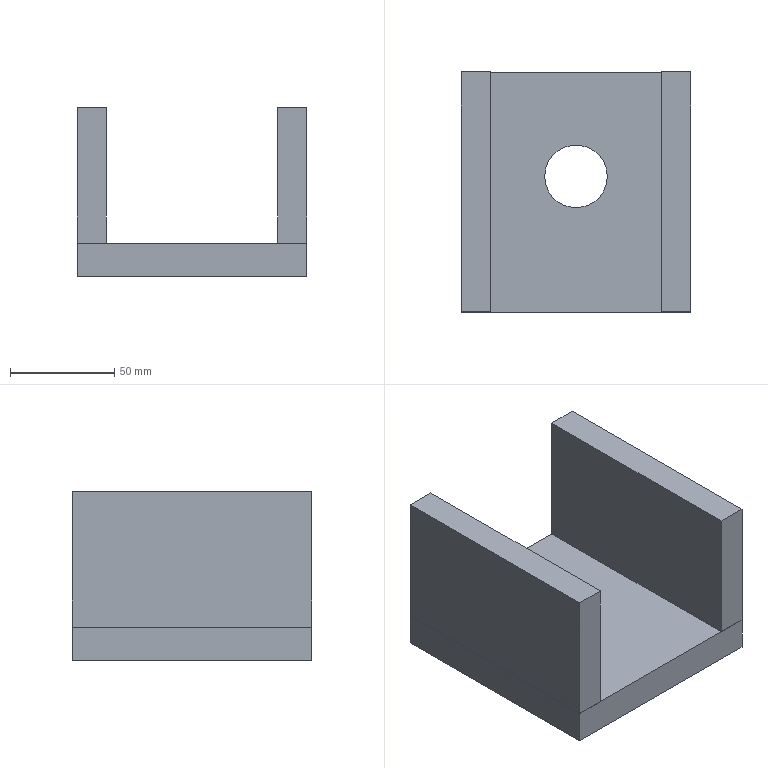Part | SolidWorks | features ICE 3, Extrusion 1, MirrorSolid 1, WeldmentFeature 1 | 3 solids | 20 faces | box 110 x 115 x 81 mm | volume 400390 mm3 | plane 18 | cylinder 2 | commonest cylinder face diameters 30 x2
STEP:
#1=CARTESIAN_POINT('',(-55.,50.,81.));
#2=VERTEX_POINT('',#1);
#3=CARTESIAN_POINT('',(-55.,50.,16.));
#4=VERTEX_POINT('',#3);
#5=CARTESIAN_POINT('',(-55.,50.,16.));
#6=DIRECTION('',(0.,0.,-1.));
#7=VECTOR('',#6,1000.);
#8=LINE('',#5,#7);
#9=EDGE_CURVE('',#2,#4,#8,.T.);
#10=ORIENTED_EDGE('',*,*,#9,.F.);
#11=CARTESIAN_POINT('',(-41.,50.,81.));
#12=VERTEX_POINT('',#11);
#13=CARTESIAN_POINT('',(-41.,50.,81.));
#14=DIRECTION('',(-1.,0.,0.));
#15=VECTOR('',#14,1000.);
#16=LINE('',#13,#15);
#17=EDGE_CURVE('',#12,#2,#16,.T.);
#18=ORIENTED_EDGE('',*,*,#17,.F.);
#19=CARTESIAN_POINT('',(-41.,50.,16.));
#20=VERTEX_POINT('',#19);
#21=CARTESIAN_POINT('',(-41.,50.,16.));
#22=DIRECTION('',(0.,0.,-1.));
#23=VECTOR('',#22,1000.);
#24=LINE('',#21,#23);
#25=EDGE_CURVE('',#12,#20,#24,.T.);
#26=ORIENTED_EDGE('',*,*,#25,.T.);
#27=CARTESIAN_POINT('',(-41.,50.,16.));
#28=DIRECTION('',(-1.,0.,0.));
#29=VECTOR('',#28,1000.);
#30=LINE('',#27,#29);
#31=EDGE_CURVE('',#20,#4,#30,.T.);
#32=ORIENTED_EDGE('',*,*,#31,.T.);
#33=EDGE_LOOP('',(#10,#18,#26,#32));
#34=FACE_OUTER_BOUND('',#33,.T.);
#35=CARTESIAN_POINT('',(-41.,50.,16.));
#36=DIRECTION('',(0.,1.,0.));
#37=DIRECTION('',(0.,0.,1.));
#38=AXIS2_PLACEMENT_3D('',#35,#36,#37);
#39=PLANE('',#38);
#40=ADVANCED_FACE('',(#34),#39,.T.);
#41=CARTESIAN_POINT('',(-55.,-65.,81.));
#42=VERTEX_POINT('',#41);
#43=CARTESIAN_POINT('',(-55.,50.,81.));
#44=DIRECTION('',(0.,1.,0.));
#45=VECTOR('',#44,1000.);
#46=LINE('',#43,#45);
#47=EDGE_CURVE('',#42,#2,#46,.T.);
#48=ORIENTED_EDGE('',*,*,#47,.F.);
#49=CARTESIAN_POINT('',(-41.,-65.,81.));
#50=VERTEX_POINT('',#49);
#51=CARTESIAN_POINT('',(-41.,-65.,81.));
#52=DIRECTION('',(-1.,0.,0.));
#53=VECTOR('',#52,1000.);
#54=LINE('',#51,#53);
#55=EDGE_CURVE('',#50,#42,#54,.T.);
#56=ORIENTED_EDGE('',*,*,#55,.F.);
#57=CARTESIAN_POINT('',(-41.,50.,81.));
#58=DIRECTION('',(0.,1.,0.));
#59=VECTOR('',#58,1000.);
#60=LINE('',#57,#59);
#61=EDGE_CURVE('',#50,#12,#60,.T.);
#62=ORIENTED_EDGE('',*,*,#61,.T.);
#63=ORIENTED_EDGE('',*,*,#17,.T.);
#64=EDGE_LOOP('',(#48,#56,#62,#63));
#65=FACE_OUTER_BOUND('',#64,.T.);
#66=CARTESIAN_POINT('',(-41.,50.,81.));
#67=DIRECTION('',(0.,0.,1.));
#68=DIRECTION('',(0.,-1.,0.));
#69=AXIS2_PLACEMENT_3D('',#66,#67,#68);
#70=PLANE('',#69);
#71=ADVANCED_FACE('',(#65),#70,.T.);
#72=CARTESIAN_POINT('',(-55.,-65.,16.));
#73=VERTEX_POINT('',#72);
#74=CARTESIAN_POINT('',(-55.,-65.,16.));
#75=DIRECTION('',(0.,0.,1.));
#76=VECTOR('',#75,1000.);
#77=LINE('',#74,#76);
#78=EDGE_CURVE('',#73,#42,#77,.T.);
#79=ORIENTED_EDGE('',*,*,#78,.F.);
#80=CARTESIAN_POINT('',(-41.,-65.,16.));
#81=VERTEX_POINT('',#80);
#82=CARTESIAN_POINT('',(-41.,-65.,16.));
#83=DIRECTION('',(-1.,0.,0.));
#84=VECTOR('',#83,1000.);
#85=LINE('',#82,#84);
#86=EDGE_CURVE('',#81,#73,#85,.T.);
#87=ORIENTED_EDGE('',*,*,#86,.F.);
#88=CARTESIAN_POINT('',(-41.,-65.,16.));
#89=DIRECTION('',(0.,0.,1.));
#90=VECTOR('',#89,1000.);
#91=LINE('',#88,#90);
#92=EDGE_CURVE('',#81,#50,#91,.T.);
#93=ORIENTED_EDGE('',*,*,#92,.T.);
#94=ORIENTED_EDGE('',*,*,#55,.T.);
#95=EDGE_LOOP('',(#79,#87,#93,#94));
#96=FACE_OUTER_BOUND('',#95,.T.);
#97=CARTESIAN_POINT('',(-41.,-65.,16.));
#98=DIRECTION('',(0.,-1.,0.));
#99=DIRECTION('',(0.,0.,-1.));
#100=AXIS2_PLACEMENT_3D('',#97,#98,#99);
#101=PLANE('',#100);
#102=ADVANCED_FACE('',(#96),#101,.T.);
#103=CARTESIAN_POINT('',(-55.,50.,16.));
#104=DIRECTION('',(0.,-1.,0.));
#105=VECTOR('',#104,1000.);
#106=LINE('',#103,#105);
#107=EDGE_CURVE('',#4,#73,#106,.T.);
#108=ORIENTED_EDGE('',*,*,#107,.F.);
#109=ORIENTED_EDGE('',*,*,#31,.F.);
#110=CARTESIAN_POINT('',(-41.,50.,16.));
#111=DIRECTION('',(0.,-1.,0.));
#112=VECTOR('',#111,1000.);
#113=LINE('',#110,#112);
#114=EDGE_CURVE('',#20,#81,#113,.T.);
#115=ORIENTED_EDGE('',*,*,#114,.T.);
#116=ORIENTED_EDGE('',*,*,#86,.T.);
#117=EDGE_LOOP('',(#108,#109,#115,#116));
#118=FACE_OUTER_BOUND('',#117,.T.);
#119=CARTESIAN_POINT('',(-41.,50.,16.));
#120=DIRECTION('',(0.,0.,-1.));
#121=DIRECTION('',(0.,1.,0.));
#122=AXIS2_PLACEMENT_3D('',#119,#120,#121);
#123=PLANE('',#122);
#124=ADVANCED_FACE('',(#118),#123,.T.);
#125=ORIENTED_EDGE('',*,*,#25,.F.);
#126=ORIENTED_EDGE('',*,*,#61,.F.);
#127=ORIENTED_EDGE('',*,*,#92,.F.);
#128=ORIENTED_EDGE('',*,*,#114,.F.);
#129=EDGE_LOOP('',(#125,#126,#127,#128));
#130=FACE_OUTER_BOUND('',#129,.T.);
#131=CARTESIAN_POINT('',(-41.,0.,0.));
#132=DIRECTION('',(1.,0.,0.));
#133=DIRECTION('',(0.,0.,-1.));
#134=AXIS2_PLACEMENT_3D('',#131,#132,#133);
#135=PLANE('',#134);
#136=ADVANCED_FACE('',(#130),#135,.T.);
#137=ORIENTED_EDGE('',*,*,#9,.T.);
#138=ORIENTED_EDGE('',*,*,#107,.T.);
#139=ORIENTED_EDGE('',*,*,#78,.T.);
#140=ORIENTED_EDGE('',*,*,#47,.T.);
#141=EDGE_LOOP('',(#137,#138,#139,#140));
#142=FACE_OUTER_BOUND('',#141,.T.);
#143=CARTESIAN_POINT('',(-55.,0.,0.));
#144=DIRECTION('',(1.,0.,0.));
#145=DIRECTION('',(0.,0.,-1.));
#146=AXIS2_PLACEMENT_3D('',#143,#144,#145);
#147=PLANE('',#146);
#148=ADVANCED_FACE('',(#142),#147,.F.);
#149=CLOSED_SHELL('',(#40,#71,#102,#124,#136,#148));
#150=MANIFOLD_SOLID_BREP('',#149);
#151=CARTESIAN_POINT('',(55.,50.,81.));
#152=VERTEX_POINT('',#151);
#153=CARTESIAN_POINT('',(55.,50.,16.));
#154=VERTEX_POINT('',#153);
#155=CARTESIAN_POINT('',(55.,50.,16.));
#156=DIRECTION('',(0.,0.,-1.));
#157=VECTOR('',#156,1000.);
#158=LINE('',#155,#157);
#159=EDGE_CURVE('',#152,#154,#158,.T.);
#160=ORIENTED_EDGE('',*,*,#159,.T.);
#161=CARTESIAN_POINT('',(41.,50.,16.));
#162=VERTEX_POINT('',#161);
#163=CARTESIAN_POINT('',(41.,50.,16.));
#164=DIRECTION('',(1.,0.,0.));
#165=VECTOR('',#164,1000.);
#166=LINE('',#163,#165);
#167=EDGE_CURVE('',#162,#154,#166,.T.);
#168=ORIENTED_EDGE('',*,*,#167,.F.);
#169=CARTESIAN_POINT('',(41.,50.,81.));
#170=VERTEX_POINT('',#169);
#171=CARTESIAN_POINT('',(41.,50.,16.));
#172=DIRECTION('',(0.,0.,-1.));
#173=VECTOR('',#172,1000.);
#174=LINE('',#171,#173);
#175=EDGE_CURVE('',#170,#162,#174,.T.);
#176=ORIENTED_EDGE('',*,*,#175,.F.);
#177=CARTESIAN_POINT('',(41.,50.,81.));
#178=DIRECTION('',(1.,0.,0.));
#179=VECTOR('',#178,1000.);
#180=LINE('',#177,#179);
#181=EDGE_CURVE('',#170,#152,#180,.T.);
#182=ORIENTED_EDGE('',*,*,#181,.T.);
#183=EDGE_LOOP('',(#160,#168,#176,#182));
#184=FACE_OUTER_BOUND('',#183,.T.);
#185=CARTESIAN_POINT('',(41.,50.,16.));
#186=DIRECTION('',(0.,1.,0.));
#187=DIRECTION('',(0.,0.,1.));
#188=AXIS2_PLACEMENT_3D('',#185,#186,#187);
#189=PLANE('',#188);
#190=ADVANCED_FACE('',(#184),#189,.T.);
#191=CARTESIAN_POINT('',(55.,-65.,81.));
#192=VERTEX_POINT('',#191);
#193=CARTESIAN_POINT('',(55.,50.,81.));
#194=DIRECTION('',(0.,1.,0.));
#195=VECTOR('',#194,1000.);
#196=LINE('',#193,#195);
#197=EDGE_CURVE('',#192,#152,#196,.T.);
#198=ORIENTED_EDGE('',*,*,#197,.T.);
#199=ORIENTED_EDGE('',*,*,#181,.F.);
#200=CARTESIAN_POINT('',(41.,-65.,81.));
#201=VERTEX_POINT('',#200);
#202=CARTESIAN_POINT('',(41.,50.,81.));
#203=DIRECTION('',(0.,1.,0.));
#204=VECTOR('',#203,1000.);
#205=LINE('',#202,#204);
#206=EDGE_CURVE('',#201,#170,#205,.T.);
#207=ORIENTED_EDGE('',*,*,#206,.F.);
#208=CARTESIAN_POINT('',(41.,-65.,81.));
#209=DIRECTION('',(1.,0.,0.));
#210=VECTOR('',#209,1000.);
#211=LINE('',#208,#210);
#212=EDGE_CURVE('',#201,#192,#211,.T.);
#213=ORIENTED_EDGE('',*,*,#212,.T.);
#214=EDGE_LOOP('',(#198,#199,#207,#213));
#215=FACE_OUTER_BOUND('',#214,.T.);
#216=CARTESIAN_POINT('',(41.,50.,81.));
#217=DIRECTION('',(0.,0.,1.));
#218=DIRECTION('',(0.,-1.,0.));
#219=AXIS2_PLACEMENT_3D('',#216,#217,#218);
#220=PLANE('',#219);
#221=ADVANCED_FACE('',(#215),#220,.T.);
#222=CARTESIAN_POINT('',(55.,-65.,16.));
#223=VERTEX_POINT('',#222);
#224=CARTESIAN_POINT('',(55.,-65.,16.));
#225=DIRECTION('',(0.,0.,1.));
#226=VECTOR('',#225,1000.);
#227=LINE('',#224,#226);
#228=EDGE_CURVE('',#223,#192,#227,.T.);
#229=ORIENTED_EDGE('',*,*,#228,.T.);
#230=ORIENTED_EDGE('',*,*,#212,.F.);
#231=CARTESIAN_POINT('',(41.,-65.,16.));
#232=VERTEX_POINT('',#231);
#233=CARTESIAN_POINT('',(41.,-65.,16.));
#234=DIRECTION('',(0.,0.,1.));
#235=VECTOR('',#234,1000.);
#236=LINE('',#233,#235);
#237=EDGE_CURVE('',#232,#201,#236,.T.);
#238=ORIENTED_EDGE('',*,*,#237,.F.);
#239=CARTESIAN_POINT('',(41.,-65.,16.));
#240=DIRECTION('',(1.,0.,0.));
#241=VECTOR('',#240,1000.);
#242=LINE('',#239,#241);
#243=EDGE_CURVE('',#232,#223,#242,.T.);
#244=ORIENTED_EDGE('',*,*,#243,.T.);
#245=EDGE_LOOP('',(#229,#230,#238,#244));
#246=FACE_OUTER_BOUND('',#245,.T.);
#247=CARTESIAN_POINT('',(41.,-65.,16.));
#248=DIRECTION('',(0.,-1.,0.));
#249=DIRECTION('',(0.,0.,-1.));
#250=AXIS2_PLACEMENT_3D('',#247,#248,#249);
#251=PLANE('',#250);
#252=ADVANCED_FACE('',(#246),#251,.T.);
#253=CARTESIAN_POINT('',(55.,50.,16.));
#254=DIRECTION('',(0.,-1.,0.));
#255=VECTOR('',#254,1000.);
#256=LINE('',#253,#255);
#257=EDGE_CURVE('',#154,#223,#256,.T.);
#258=ORIENTED_EDGE('',*,*,#257,.T.);
#259=ORIENTED_EDGE('',*,*,#243,.F.);
#260=CARTESIAN_POINT('',(41.,50.,16.));
#261=DIRECTION('',(0.,-1.,0.));
#262=VECTOR('',#261,1000.);
#263=LINE('',#260,#262);
#264=EDGE_CURVE('',#162,#232,#263,.T.);
#265=ORIENTED_EDGE('',*,*,#264,.F.);
#266=ORIENTED_EDGE('',*,*,#167,.T.);
#267=EDGE_LOOP('',(#258,#259,#265,#266));
#268=FACE_OUTER_BOUND('',#267,.T.);
#269=CARTESIAN_POINT('',(41.,50.,16.));
#270=DIRECTION('',(0.,0.,-1.));
#271=DIRECTION('',(0.,1.,0.));
#272=AXIS2_PLACEMENT_3D('',#269,#270,#271);
#273=PLANE('',#272);
#274=ADVANCED_FACE('',(#268),#273,.T.);
#275=ORIENTED_EDGE('',*,*,#175,.T.);
#276=ORIENTED_EDGE('',*,*,#264,.T.);
#277=ORIENTED_EDGE('',*,*,#237,.T.);
#278=ORIENTED_EDGE('',*,*,#206,.T.);
#279=EDGE_LOOP('',(#275,#276,#277,#278));
#280=FACE_OUTER_BOUND('',#279,.T.);
#281=CARTESIAN_POINT('',(41.,0.,0.));
#282=DIRECTION('',(-1.,0.,0.));
#283=DIRECTION('',(0.,0.,-1.));
#284=AXIS2_PLACEMENT_3D('',#281,#282,#283);
#285=PLANE('',#284);
#286=ADVANCED_FACE('',(#280),#285,.T.);
#287=ORIENTED_EDGE('',*,*,#159,.F.);
#288=ORIENTED_EDGE('',*,*,#197,.F.);
#289=ORIENTED_EDGE('',*,*,#228,.F.);
#290=ORIENTED_EDGE('',*,*,#257,.F.);
#291=EDGE_LOOP('',(#287,#288,#289,#290));
#292=FACE_OUTER_BOUND('',#291,.T.);
#293=CARTESIAN_POINT('',(55.,0.,0.));
#294=DIRECTION('',(-1.,0.,0.));
#295=DIRECTION('',(0.,0.,-1.));
#296=AXIS2_PLACEMENT_3D('',#293,#294,#295);
#297=PLANE('',#296);
#298=ADVANCED_FACE('',(#292),#297,.F.);
#299=CLOSED_SHELL('',(#190,#221,#252,#274,#286,#298));
#300=MANIFOLD_SOLID_BREP('',#299);
#301=CARTESIAN_POINT('',(-15.,0.,16.));
#302=VERTEX_POINT('',#301);
#303=CARTESIAN_POINT('',(15.,0.,16.));
#304=VERTEX_POINT('',#303);
#305=CARTESIAN_POINT('',(0.,0.,16.));
#306=DIRECTION('',(0.,0.,1.));
#307=DIRECTION('',(-1.,0.,0.));
#308=AXIS2_PLACEMENT_3D('',#305,#306,#307);
#309=CIRCLE('',#308,15.);
#310=EDGE_CURVE('',#302,#304,#309,.T.);
#311=ORIENTED_EDGE('',*,*,#310,.T.);
#312=CARTESIAN_POINT('',(15.,0.,0.));
#313=VERTEX_POINT('',#312);
#314=CARTESIAN_POINT('',(15.,0.,81.001));
#315=DIRECTION('',(0.,0.,-1.));
#316=VECTOR('',#315,1000.);
#317=LINE('',#314,#316);
#318=EDGE_CURVE('',#304,#313,#317,.T.);
#319=ORIENTED_EDGE('',*,*,#318,.T.);
#320=CARTESIAN_POINT('',(-15.,0.,0.));
#321=VERTEX_POINT('',#320);
#322=CARTESIAN_POINT('',(0.,0.,0.));
#323=DIRECTION('',(0.,0.,-1.));
#324=DIRECTION('',(-1.,0.,0.));
#325=AXIS2_PLACEMENT_3D('',#322,#323,#324);
#326=CIRCLE('',#325,15.);
#327=EDGE_CURVE('',#313,#321,#326,.T.);
#328=ORIENTED_EDGE('',*,*,#327,.T.);
#329=CARTESIAN_POINT('',(-15.,0.,81.001));
#330=DIRECTION('',(0.,0.,-1.));
#331=VECTOR('',#330,1000.);
#332=LINE('',#329,#331);
#333=EDGE_CURVE('',#302,#321,#332,.T.);
#334=ORIENTED_EDGE('',*,*,#333,.F.);
#335=EDGE_LOOP('',(#311,#319,#328,#334));
#336=FACE_OUTER_BOUND('',#335,.T.);
#337=CARTESIAN_POINT('',(0.,0.,81.001));
#338=DIRECTION('',(0.,0.,-1.));
#339=DIRECTION('',(-1.,0.,0.));
#340=AXIS2_PLACEMENT_3D('',#337,#338,#339);
#341=CYLINDRICAL_SURFACE('',#340,15.);
#342=ADVANCED_FACE('',(#336),#341,.F.);
#343=CARTESIAN_POINT('',(55.,-65.,0.));
#344=VERTEX_POINT('',#343);
#345=CARTESIAN_POINT('',(55.,50.,0.));
#346=VERTEX_POINT('',#345);
#347=CARTESIAN_POINT('',(55.,-50.,0.));
#348=DIRECTION('',(0.,1.,0.));
#349=VECTOR('',#348,1000.);
#350=LINE('',#347,#349);
#351=EDGE_CURVE('',#344,#346,#350,.T.);
#352=ORIENTED_EDGE('',*,*,#351,.T.);
#353=CARTESIAN_POINT('',(55.,50.,16.));
#354=VERTEX_POINT('',#353);
#355=CARTESIAN_POINT('',(55.,50.,16.));
#356=DIRECTION('',(0.,0.,-1.));
#357=VECTOR('',#356,1000.);
#358=LINE('',#355,#357);
#359=EDGE_CURVE('',#354,#346,#358,.T.);
#360=ORIENTED_EDGE('',*,*,#359,.F.);
#361=CARTESIAN_POINT('',(55.,-65.,16.));
#362=VERTEX_POINT('',#361);
#363=CARTESIAN_POINT('',(55.,-50.,16.));
#364=DIRECTION('',(0.,1.,0.));
#365=VECTOR('',#364,1000.);
#366=LINE('',#363,#365);
#367=EDGE_CURVE('',#362,#354,#366,.T.);
#368=ORIENTED_EDGE('',*,*,#367,.F.);
#369=CARTESIAN_POINT('',(55.,-65.,16.));
#370=DIRECTION('',(0.,0.,1.));
#371=VECTOR('',#370,1000.);
#372=LINE('',#369,#371);
#373=EDGE_CURVE('',#344,#362,#372,.T.);
#374=ORIENTED_EDGE('',*,*,#373,.F.);
#375=EDGE_LOOP('',(#352,#360,#368,#374));
#376=FACE_OUTER_BOUND('',#375,.T.);
#377=CARTESIAN_POINT('',(55.,-50.,16.));
#378=DIRECTION('',(-1.,0.,0.));
#379=DIRECTION('',(0.,0.,1.));
#380=AXIS2_PLACEMENT_3D('',#377,#378,#379);
#381=PLANE('',#380);
#382=ADVANCED_FACE('',(#376),#381,.F.);
#383=CARTESIAN_POINT('',(-55.,50.,0.));
#384=VERTEX_POINT('',#383);
#385=CARTESIAN_POINT('',(-55.,50.,0.));
#386=DIRECTION('',(-1.,0.,0.));
#387=VECTOR('',#386,1000.);
#388=LINE('',#385,#387);
#389=EDGE_CURVE('',#346,#384,#388,.T.);
#390=ORIENTED_EDGE('',*,*,#389,.T.);
#391=CARTESIAN_POINT('',(-55.,50.,16.));
#392=VERTEX_POINT('',#391);
#393=CARTESIAN_POINT('',(-55.,50.,16.));
#394=DIRECTION('',(0.,0.,-1.));
#395=VECTOR('',#394,1000.);
#396=LINE('',#393,#395);
#397=EDGE_CURVE('',#392,#384,#396,.T.);
#398=ORIENTED_EDGE('',*,*,#397,.F.);
#399=CARTESIAN_POINT('',(-55.,50.,16.));
#400=DIRECTION('',(-1.,0.,0.));
#401=VECTOR('',#400,1000.);
#402=LINE('',#399,#401);
#403=EDGE_CURVE('',#354,#392,#402,.T.);
#404=ORIENTED_EDGE('',*,*,#403,.F.);
#405=ORIENTED_EDGE('',*,*,#359,.T.);
#406=EDGE_LOOP('',(#390,#398,#404,#405));
#407=FACE_OUTER_BOUND('',#406,.T.);
#408=CARTESIAN_POINT('',(-55.,50.,16.));
#409=DIRECTION('',(0.,-1.,0.));
#410=DIRECTION('',(0.,0.,-1.));
#411=AXIS2_PLACEMENT_3D('',#408,#409,#410);
#412=PLANE('',#411);
#413=ADVANCED_FACE('',(#407),#412,.F.);
#414=CARTESIAN_POINT('',(-55.,-65.,0.));
#415=VERTEX_POINT('',#414);
#416=CARTESIAN_POINT('',(-55.,-50.,0.));
#417=DIRECTION('',(0.,-1.,0.));
#418=VECTOR('',#417,1000.);
#419=LINE('',#416,#418);
#420=EDGE_CURVE('',#384,#415,#419,.T.);
#421=ORIENTED_EDGE('',*,*,#420,.T.);
#422=CARTESIAN_POINT('',(-55.,-65.,16.));
#423=VERTEX_POINT('',#422);
#424=CARTESIAN_POINT('',(-55.,-65.,16.));
#425=DIRECTION('',(0.,0.,-1.));
#426=VECTOR('',#425,1000.);
#427=LINE('',#424,#426);
#428=EDGE_CURVE('',#423,#415,#427,.T.);
#429=ORIENTED_EDGE('',*,*,#428,.F.);
#430=CARTESIAN_POINT('',(-55.,-50.,16.));
#431=DIRECTION('',(0.,-1.,0.));
#432=VECTOR('',#431,1000.);
#433=LINE('',#430,#432);
#434=EDGE_CURVE('',#392,#423,#433,.T.);
#435=ORIENTED_EDGE('',*,*,#434,.F.);
#436=ORIENTED_EDGE('',*,*,#397,.T.);
#437=EDGE_LOOP('',(#421,#429,#435,#436));
#438=FACE_OUTER_BOUND('',#437,.T.);
#439=CARTESIAN_POINT('',(-55.,-50.,16.));
#440=DIRECTION('',(1.,0.,0.));
#441=DIRECTION('',(0.,0.,-1.));
#442=AXIS2_PLACEMENT_3D('',#439,#440,#441);
#443=PLANE('',#442);
#444=ADVANCED_FACE('',(#438),#443,.F.);
#445=ORIENTED_EDGE('',*,*,#310,.F.);
#446=CARTESIAN_POINT('',(0.,0.,16.));
#447=DIRECTION('',(0.,0.,1.));
#448=DIRECTION('',(-1.,0.,0.));
#449=AXIS2_PLACEMENT_3D('',#446,#447,#448);
#450=CIRCLE('',#449,15.);
#451=EDGE_CURVE('',#304,#302,#450,.T.);
#452=ORIENTED_EDGE('',*,*,#451,.F.);
#453=EDGE_LOOP('',(#445,#452));
#454=FACE_BOUND('',#453,.T.);
#455=ORIENTED_EDGE('',*,*,#367,.T.);
#456=ORIENTED_EDGE('',*,*,#403,.T.);
#457=ORIENTED_EDGE('',*,*,#434,.T.);
#458=CARTESIAN_POINT('',(-55.,-65.,16.));
#459=DIRECTION('',(-1.,0.,0.));
#460=VECTOR('',#459,1000.);
#461=LINE('',#458,#460);
#462=EDGE_CURVE('',#362,#423,#461,.T.);
#463=ORIENTED_EDGE('',*,*,#462,.F.);
#464=EDGE_LOOP('',(#455,#456,#457,#463));
#465=FACE_OUTER_BOUND('',#464,.T.);
#466=CARTESIAN_POINT('',(0.,0.,16.));
#467=DIRECTION('',(0.,0.,-1.));
#468=DIRECTION('',(-1.,0.,0.));
#469=AXIS2_PLACEMENT_3D('',#466,#467,#468);
#470=PLANE('',#469);
#471=ADVANCED_FACE('',(#454,#465),#470,.F.);
#472=CARTESIAN_POINT('',(0.,0.,0.));
#473=DIRECTION('',(0.,0.,-1.));
#474=DIRECTION('',(-1.,0.,0.));
#475=AXIS2_PLACEMENT_3D('',#472,#473,#474);
#476=CIRCLE('',#475,15.);
#477=EDGE_CURVE('',#321,#313,#476,.T.);
#478=ORIENTED_EDGE('',*,*,#477,.F.);
#479=ORIENTED_EDGE('',*,*,#327,.F.);
#480=EDGE_LOOP('',(#478,#479));
#481=FACE_BOUND('',#480,.T.);
#482=ORIENTED_EDGE('',*,*,#351,.F.);
#483=CARTESIAN_POINT('',(-55.,-65.,0.));
#484=DIRECTION('',(1.,0.,0.));
#485=VECTOR('',#484,1000.);
#486=LINE('',#483,#485);
#487=EDGE_CURVE('',#415,#344,#486,.T.);
#488=ORIENTED_EDGE('',*,*,#487,.F.);
#489=ORIENTED_EDGE('',*,*,#420,.F.);
#490=ORIENTED_EDGE('',*,*,#389,.F.);
#491=EDGE_LOOP('',(#482,#488,#489,#490));
#492=FACE_OUTER_BOUND('',#491,.T.);
#493=CARTESIAN_POINT('',(0.,0.,0.));
#494=DIRECTION('',(0.,0.,-1.));
#495=DIRECTION('',(-1.,0.,0.));
#496=AXIS2_PLACEMENT_3D('',#493,#494,#495);
#497=PLANE('',#496);
#498=ADVANCED_FACE('',(#481,#492),#497,.T.);
#499=ORIENTED_EDGE('',*,*,#318,.F.);
#500=ORIENTED_EDGE('',*,*,#451,.T.);
#501=ORIENTED_EDGE('',*,*,#333,.T.);
#502=ORIENTED_EDGE('',*,*,#477,.T.);
#503=EDGE_LOOP('',(#499,#500,#501,#502));
#504=FACE_OUTER_BOUND('',#503,.T.);
#505=CARTESIAN_POINT('',(0.,0.,81.001));
#506=DIRECTION('',(0.,0.,-1.));
#507=DIRECTION('',(-1.,0.,0.));
#508=AXIS2_PLACEMENT_3D('',#505,#506,#507);
#509=CYLINDRICAL_SURFACE('',#508,15.);
#510=ADVANCED_FACE('',(#504),#509,.F.);
#511=ORIENTED_EDGE('',*,*,#462,.T.);
#512=ORIENTED_EDGE('',*,*,#428,.T.);
#513=ORIENTED_EDGE('',*,*,#487,.T.);
#514=ORIENTED_EDGE('',*,*,#373,.T.);
#515=EDGE_LOOP('',(#511,#512,#513,#514));
#516=FACE_OUTER_BOUND('',#515,.T.);
#517=CARTESIAN_POINT('',(-41.,-65.,16.));
#518=DIRECTION('',(0.,-1.,0.));
#519=DIRECTION('',(0.,0.,-1.));
#520=AXIS2_PLACEMENT_3D('',#517,#518,#519);
#521=PLANE('',#520);
#522=ADVANCED_FACE('',(#516),#521,.T.);
#523=CLOSED_SHELL('',(#342,#382,#413,#444,#471,#498,#510,#522));
#524=MANIFOLD_SOLID_BREP('',#523);
#525=CARTESIAN_POINT('',(0.,0.,0.));
#526=DIRECTION('',(0.,0.,1.));
#527=DIRECTION('',(1.,0.,0.));
#528=AXIS2_PLACEMENT_3D('',#525,#526,#527);
#529=(LENGTH_UNIT()NAMED_UNIT(*)SI_UNIT(.MILLI.,.METRE.));
#530=UNCERTAINTY_MEASURE_WITH_UNIT(LENGTH_MEASURE(0.00001),#529,'','');
#531=(NAMED_UNIT(*)PLANE_ANGLE_UNIT()SI_UNIT($,.RADIAN.));
#532=(NAMED_UNIT(*)SI_UNIT($,.STERADIAN.)SOLID_ANGLE_UNIT());
#533=(GEOMETRIC_REPRESENTATION_CONTEXT(3)GLOBAL_UNCERTAINTY_ASSIGNED_CONTEXT((#530))GLOBAL_UNIT_ASSIGNED_CONTEXT((#529,#531,#532))REPRESENTATION_CONTEXT('',''));
#534=ADVANCED_BREP_SHAPE_REPRESENTATION('',(#150,#300,#524,#528),#533);